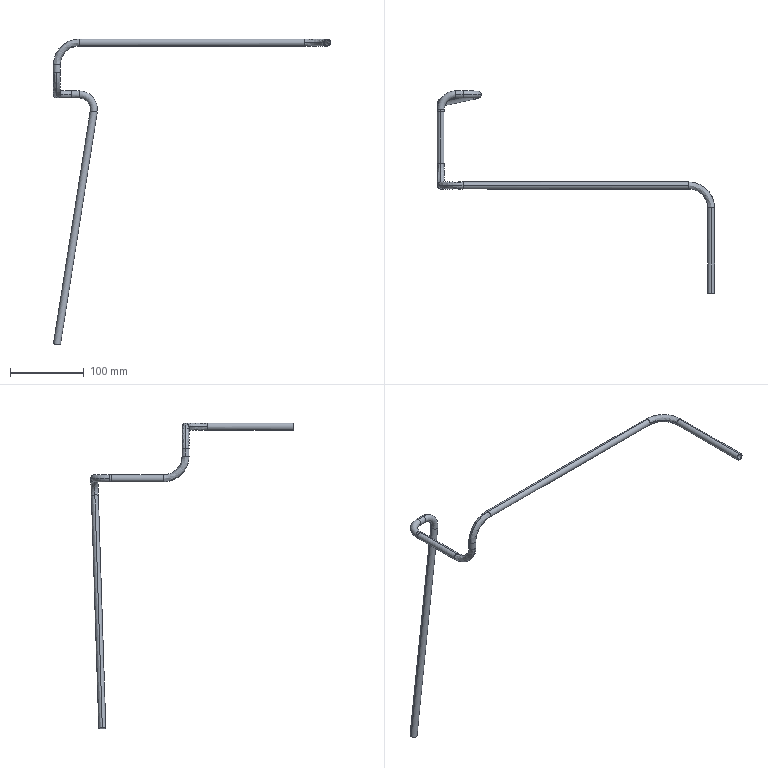Part | STEP file | copper tube 25_default_machined_ | 2 solids | 42 faces | box 374.675 x 273.558 x 413.267 mm | volume 42436 mm3 | cylinder 22 | spline 12 | plane 4 | torus 4 | commonest cylinder face diameters 9.525 x14 7.925 x8